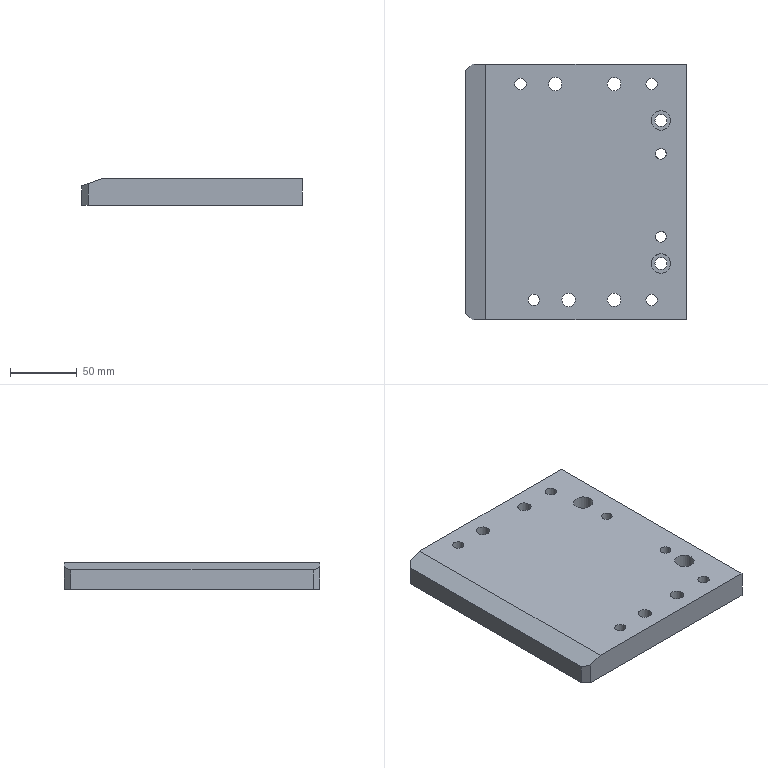Part | NX | features DIE-1 2 | 1 solid | 25 faces | box 165 x 191 x 20 mm | volume 604511 mm3 | cylinder 14 | plane 11 | commonest cylinder face diameters 8.506 x4 10 x4 8 x2 9.007 x2 14.5 x2
STEP:
#1=CARTESIAN_POINT('',(2183.347,-939.822,858.716));
#2=VERTEX_POINT('',#1);
#3=CARTESIAN_POINT('',(2179.094,-939.822,858.716));
#4=DIRECTION('',(0.,0.,-1.));
#5=DIRECTION('',(1.,0.,0.));
#6=AXIS2_PLACEMENT_3D('',#3,#4,#5);
#7=CIRCLE('',#6,4.253);
#8=EDGE_CURVE('',#2,#2,#7,.T.);
#9=ORIENTED_EDGE('',*,*,#8,.T.);
#10=EDGE_LOOP('',(#9));
#11=FACE_BOUND('',#10,.T.);
#12=CARTESIAN_POINT('',(2210.094,-939.822,858.716));
#13=VERTEX_POINT('',#12);
#14=CARTESIAN_POINT('',(2205.094,-939.822,858.716));
#15=DIRECTION('',(0.,0.,-1.));
#16=DIRECTION('',(1.,0.,0.));
#17=AXIS2_PLACEMENT_3D('',#14,#15,#16);
#18=CIRCLE('',#17,5.);
#19=EDGE_CURVE('',#13,#13,#18,.T.);
#20=ORIENTED_EDGE('',*,*,#19,.T.);
#21=EDGE_LOOP('',(#20));
#22=FACE_BOUND('',#21,.T.);
#23=CARTESIAN_POINT('',(2271.347,-939.822,858.716));
#24=VERTEX_POINT('',#23);
#25=CARTESIAN_POINT('',(2267.094,-939.822,858.716));
#26=DIRECTION('',(0.,0.,-1.));
#27=DIRECTION('',(1.,0.,0.));
#28=AXIS2_PLACEMENT_3D('',#25,#26,#27);
#29=CIRCLE('',#28,4.253);
#30=EDGE_CURVE('',#24,#24,#29,.T.);
#31=ORIENTED_EDGE('',*,*,#30,.T.);
#32=EDGE_LOOP('',(#31));
#33=FACE_BOUND('',#32,.T.);
#34=CARTESIAN_POINT('',(2244.094,-939.822,858.716));
#35=VERTEX_POINT('',#34);
#36=CARTESIAN_POINT('',(2239.094,-939.822,858.716));
#37=DIRECTION('',(0.,0.,-1.));
#38=DIRECTION('',(1.,0.,0.));
#39=AXIS2_PLACEMENT_3D('',#36,#37,#38);
#40=CIRCLE('',#39,5.);
#41=EDGE_CURVE('',#35,#35,#40,.T.);
#42=ORIENTED_EDGE('',*,*,#41,.T.);
#43=EDGE_LOOP('',(#42));
#44=FACE_BOUND('',#43,.T.);
#45=CARTESIAN_POINT('',(2173.347,-778.422,858.716));
#46=VERTEX_POINT('',#45);
#47=CARTESIAN_POINT('',(2169.094,-778.422,858.716));
#48=DIRECTION('',(0.,0.,-1.));
#49=DIRECTION('',(1.,0.,0.));
#50=AXIS2_PLACEMENT_3D('',#47,#48,#49);
#51=CIRCLE('',#50,4.253);
#52=EDGE_CURVE('',#46,#46,#51,.T.);
#53=ORIENTED_EDGE('',*,*,#52,.T.);
#54=EDGE_LOOP('',(#53));
#55=FACE_BOUND('',#54,.T.);
#56=CARTESIAN_POINT('',(2271.347,-778.422,858.716));
#57=VERTEX_POINT('',#56);
#58=CARTESIAN_POINT('',(2267.094,-778.422,858.716));
#59=DIRECTION('',(0.,0.,-1.));
#60=DIRECTION('',(1.,0.,0.));
#61=AXIS2_PLACEMENT_3D('',#58,#59,#60);
#62=CIRCLE('',#61,4.253);
#63=EDGE_CURVE('',#57,#57,#62,.T.);
#64=ORIENTED_EDGE('',*,*,#63,.T.);
#65=EDGE_LOOP('',(#64));
#66=FACE_BOUND('',#65,.T.);
#67=CARTESIAN_POINT('',(2200.094,-778.422,858.716));
#68=VERTEX_POINT('',#67);
#69=CARTESIAN_POINT('',(2195.094,-778.422,858.716));
#70=DIRECTION('',(0.,0.,-1.));
#71=DIRECTION('',(1.,0.,0.));
#72=AXIS2_PLACEMENT_3D('',#69,#70,#71);
#73=CIRCLE('',#72,5.);
#74=EDGE_CURVE('',#68,#68,#73,.T.);
#75=ORIENTED_EDGE('',*,*,#74,.T.);
#76=EDGE_LOOP('',(#75));
#77=FACE_BOUND('',#76,.T.);
#78=CARTESIAN_POINT('',(2244.094,-778.422,858.716));
#79=VERTEX_POINT('',#78);
#80=CARTESIAN_POINT('',(2239.094,-778.422,858.716));
#81=DIRECTION('',(0.,0.,-1.));
#82=DIRECTION('',(1.,0.,0.));
#83=AXIS2_PLACEMENT_3D('',#80,#81,#82);
#84=CIRCLE('',#83,5.);
#85=EDGE_CURVE('',#79,#79,#84,.T.);
#86=ORIENTED_EDGE('',*,*,#85,.T.);
#87=EDGE_LOOP('',(#86));
#88=FACE_BOUND('',#87,.T.);
#89=CARTESIAN_POINT('',(2281.344,-912.622,858.716));
#90=VERTEX_POINT('',#89);
#91=CARTESIAN_POINT('',(2274.094,-912.622,858.716));
#92=DIRECTION('',(0.,0.,1.));
#93=DIRECTION('',(1.,0.,0.));
#94=AXIS2_PLACEMENT_3D('',#91,#92,#93);
#95=CIRCLE('',#94,7.25);
#96=EDGE_CURVE('',#90,#90,#95,.F.);
#97=ORIENTED_EDGE('',*,*,#96,.T.);
#98=EDGE_LOOP('',(#97));
#99=FACE_BOUND('',#98,.T.);
#100=CARTESIAN_POINT('',(2278.094,-892.622,858.716));
#101=VERTEX_POINT('',#100);
#102=CARTESIAN_POINT('',(2274.094,-892.622,858.716));
#103=DIRECTION('',(0.,0.,-1.));
#104=DIRECTION('',(1.,0.,0.));
#105=AXIS2_PLACEMENT_3D('',#102,#103,#104);
#106=CIRCLE('',#105,4.);
#107=EDGE_CURVE('',#101,#101,#106,.T.);
#108=ORIENTED_EDGE('',*,*,#107,.T.);
#109=EDGE_LOOP('',(#108));
#110=FACE_BOUND('',#109,.T.);
#111=CARTESIAN_POINT('',(2278.094,-830.622,858.716));
#112=VERTEX_POINT('',#111);
#113=CARTESIAN_POINT('',(2274.094,-830.622,858.716));
#114=DIRECTION('',(0.,0.,-1.));
#115=DIRECTION('',(1.,0.,0.));
#116=AXIS2_PLACEMENT_3D('',#113,#114,#115);
#117=CIRCLE('',#116,4.);
#118=EDGE_CURVE('',#112,#112,#117,.T.);
#119=ORIENTED_EDGE('',*,*,#118,.T.);
#120=EDGE_LOOP('',(#119));
#121=FACE_BOUND('',#120,.T.);
#122=CARTESIAN_POINT('',(2281.344,-805.622,858.716));
#123=VERTEX_POINT('',#122);
#124=CARTESIAN_POINT('',(2274.094,-805.622,858.716));
#125=DIRECTION('',(0.,0.,1.));
#126=DIRECTION('',(1.,0.,0.));
#127=AXIS2_PLACEMENT_3D('',#124,#125,#126);
#128=CIRCLE('',#127,7.25);
#129=EDGE_CURVE('',#123,#123,#128,.F.);
#130=ORIENTED_EDGE('',*,*,#129,.T.);
#131=EDGE_LOOP('',(#130));
#132=FACE_BOUND('',#131,.T.);
#133=CARTESIAN_POINT('',(2293.094,-954.622,858.716));
#134=VERTEX_POINT('',#133);
#135=CARTESIAN_POINT('',(2143.094,-954.622,858.716));
#136=VERTEX_POINT('',#135);
#137=CARTESIAN_POINT('',(2118.094,-954.622,858.716));
#138=DIRECTION('',(-1.,0.,0.));
#139=VECTOR('',#138,1000.);
#140=LINE('',#137,#139);
#141=EDGE_CURVE('',#134,#136,#140,.T.);
#142=ORIENTED_EDGE('',*,*,#141,.F.);
#143=CARTESIAN_POINT('',(2293.094,-763.622,858.716));
#144=VERTEX_POINT('',#143);
#145=CARTESIAN_POINT('',(2293.094,-744.322,858.716));
#146=DIRECTION('',(0.,-1.,0.));
#147=VECTOR('',#146,1000.);
#148=LINE('',#145,#147);
#149=EDGE_CURVE('',#144,#134,#148,.T.);
#150=ORIENTED_EDGE('',*,*,#149,.F.);
#151=CARTESIAN_POINT('',(2143.094,-763.622,858.716));
#152=VERTEX_POINT('',#151);
#153=CARTESIAN_POINT('',(2293.094,-763.622,858.716));
#154=DIRECTION('',(1.,0.,0.));
#155=VECTOR('',#154,1000.);
#156=LINE('',#153,#155);
#157=EDGE_CURVE('',#152,#144,#156,.T.);
#158=ORIENTED_EDGE('',*,*,#157,.F.);
#159=CARTESIAN_POINT('',(2143.094,-830.822,858.716));
#160=DIRECTION('',(0.,-1.,0.));
#161=VECTOR('',#160,1000.);
#162=LINE('',#159,#161);
#163=EDGE_CURVE('',#152,#136,#162,.T.);
#164=ORIENTED_EDGE('',*,*,#163,.T.);
#165=EDGE_LOOP('',(#142,#150,#158,#164));
#166=FACE_BOUND('',#165,.T.);
#167=CARTESIAN_POINT('',(2203.862,-830.822,858.716));
#168=DIRECTION('',(0.,0.,1.));
#169=DIRECTION('',(-1.,0.,0.));
#170=AXIS2_PLACEMENT_3D('',#167,#168,#169);
#171=PLANE('',#170);
#172=ADVANCED_FACE('',(#11,#22,#33,#44,#55,#66,#77,#88,#99,#110,#121,#132,#166),#171,.T.);
#173=CARTESIAN_POINT('',(2183.347,-939.822,838.716));
#174=VERTEX_POINT('',#173);
#175=CARTESIAN_POINT('',(2179.094,-939.822,838.716));
#176=DIRECTION('',(0.,0.,1.));
#177=DIRECTION('',(1.,0.,0.));
#178=AXIS2_PLACEMENT_3D('',#175,#176,#177);
#179=CIRCLE('',#178,4.253);
#180=EDGE_CURVE('',#174,#174,#179,.T.);
#181=ORIENTED_EDGE('',*,*,#180,.T.);
#182=EDGE_LOOP('',(#181));
#183=FACE_BOUND('',#182,.T.);
#184=CARTESIAN_POINT('',(2210.094,-939.822,838.716));
#185=VERTEX_POINT('',#184);
#186=CARTESIAN_POINT('',(2205.094,-939.822,838.716));
#187=DIRECTION('',(0.,0.,1.));
#188=DIRECTION('',(1.,0.,0.));
#189=AXIS2_PLACEMENT_3D('',#186,#187,#188);
#190=CIRCLE('',#189,5.);
#191=EDGE_CURVE('',#185,#185,#190,.T.);
#192=ORIENTED_EDGE('',*,*,#191,.T.);
#193=EDGE_LOOP('',(#192));
#194=FACE_BOUND('',#193,.T.);
#195=CARTESIAN_POINT('',(2271.347,-939.822,838.716));
#196=VERTEX_POINT('',#195);
#197=CARTESIAN_POINT('',(2267.094,-939.822,838.716));
#198=DIRECTION('',(0.,0.,1.));
#199=DIRECTION('',(1.,0.,0.));
#200=AXIS2_PLACEMENT_3D('',#197,#198,#199);
#201=CIRCLE('',#200,4.253);
#202=EDGE_CURVE('',#196,#196,#201,.T.);
#203=ORIENTED_EDGE('',*,*,#202,.T.);
#204=EDGE_LOOP('',(#203));
#205=FACE_BOUND('',#204,.T.);
#206=CARTESIAN_POINT('',(2244.094,-939.822,838.716));
#207=VERTEX_POINT('',#206);
#208=CARTESIAN_POINT('',(2239.094,-939.822,838.716));
#209=DIRECTION('',(0.,0.,1.));
#210=DIRECTION('',(1.,0.,0.));
#211=AXIS2_PLACEMENT_3D('',#208,#209,#210);
#212=CIRCLE('',#211,5.);
#213=EDGE_CURVE('',#207,#207,#212,.T.);
#214=ORIENTED_EDGE('',*,*,#213,.T.);
#215=EDGE_LOOP('',(#214));
#216=FACE_BOUND('',#215,.T.);
#217=CARTESIAN_POINT('',(2173.347,-778.422,838.716));
#218=VERTEX_POINT('',#217);
#219=CARTESIAN_POINT('',(2169.094,-778.422,838.716));
#220=DIRECTION('',(0.,0.,1.));
#221=DIRECTION('',(1.,0.,0.));
#222=AXIS2_PLACEMENT_3D('',#219,#220,#221);
#223=CIRCLE('',#222,4.253);
#224=EDGE_CURVE('',#218,#218,#223,.T.);
#225=ORIENTED_EDGE('',*,*,#224,.T.);
#226=EDGE_LOOP('',(#225));
#227=FACE_BOUND('',#226,.T.);
#228=CARTESIAN_POINT('',(2271.347,-778.422,838.716));
#229=VERTEX_POINT('',#228);
#230=CARTESIAN_POINT('',(2267.094,-778.422,838.716));
#231=DIRECTION('',(0.,0.,1.));
#232=DIRECTION('',(1.,0.,0.));
#233=AXIS2_PLACEMENT_3D('',#230,#231,#232);
#234=CIRCLE('',#233,4.253);
#235=EDGE_CURVE('',#229,#229,#234,.T.);
#236=ORIENTED_EDGE('',*,*,#235,.T.);
#237=EDGE_LOOP('',(#236));
#238=FACE_BOUND('',#237,.T.);
#239=CARTESIAN_POINT('',(2200.094,-778.422,838.716));
#240=VERTEX_POINT('',#239);
#241=CARTESIAN_POINT('',(2195.094,-778.422,838.716));
#242=DIRECTION('',(0.,0.,1.));
#243=DIRECTION('',(1.,0.,0.));
#244=AXIS2_PLACEMENT_3D('',#241,#242,#243);
#245=CIRCLE('',#244,5.);
#246=EDGE_CURVE('',#240,#240,#245,.T.);
#247=ORIENTED_EDGE('',*,*,#246,.T.);
#248=EDGE_LOOP('',(#247));
#249=FACE_BOUND('',#248,.T.);
#250=CARTESIAN_POINT('',(2244.094,-778.422,838.716));
#251=VERTEX_POINT('',#250);
#252=CARTESIAN_POINT('',(2239.094,-778.422,838.716));
#253=DIRECTION('',(0.,0.,1.));
#254=DIRECTION('',(1.,0.,0.));
#255=AXIS2_PLACEMENT_3D('',#252,#253,#254);
#256=CIRCLE('',#255,5.);
#257=EDGE_CURVE('',#251,#251,#256,.T.);
#258=ORIENTED_EDGE('',*,*,#257,.T.);
#259=EDGE_LOOP('',(#258));
#260=FACE_BOUND('',#259,.T.);
#261=CARTESIAN_POINT('',(2278.597,-912.622,838.716));
#262=VERTEX_POINT('',#261);
#263=CARTESIAN_POINT('',(2274.094,-912.622,838.716));
#264=DIRECTION('',(0.,0.,1.));
#265=DIRECTION('',(1.,0.,0.));
#266=AXIS2_PLACEMENT_3D('',#263,#264,#265);
#267=CIRCLE('',#266,4.503);
#268=EDGE_CURVE('',#262,#262,#267,.F.);
#269=ORIENTED_EDGE('',*,*,#268,.F.);
#270=EDGE_LOOP('',(#269));
#271=FACE_BOUND('',#270,.T.);
#272=CARTESIAN_POINT('',(2274.094,-888.622,838.716));
#273=VERTEX_POINT('',#272);
#274=CARTESIAN_POINT('',(2274.094,-892.622,838.716));
#275=DIRECTION('',(0.,0.,-1.));
#276=DIRECTION('',(0.,1.,0.));
#277=AXIS2_PLACEMENT_3D('',#274,#275,#276);
#278=CIRCLE('',#277,4.);
#279=EDGE_CURVE('',#273,#273,#278,.T.);
#280=ORIENTED_EDGE('',*,*,#279,.F.);
#281=EDGE_LOOP('',(#280));
#282=FACE_BOUND('',#281,.T.);
#283=CARTESIAN_POINT('',(2274.094,-826.622,838.716));
#284=VERTEX_POINT('',#283);
#285=CARTESIAN_POINT('',(2274.094,-830.622,838.716));
#286=DIRECTION('',(0.,0.,-1.));
#287=DIRECTION('',(0.,1.,0.));
#288=AXIS2_PLACEMENT_3D('',#285,#286,#287);
#289=CIRCLE('',#288,4.);
#290=EDGE_CURVE('',#284,#284,#289,.T.);
#291=ORIENTED_EDGE('',*,*,#290,.F.);
#292=EDGE_LOOP('',(#291));
#293=FACE_BOUND('',#292,.T.);
#294=CARTESIAN_POINT('',(2278.597,-805.622,838.716));
#295=VERTEX_POINT('',#294);
#296=CARTESIAN_POINT('',(2274.094,-805.622,838.716));
#297=DIRECTION('',(0.,0.,1.));
#298=DIRECTION('',(1.,0.,0.));
#299=AXIS2_PLACEMENT_3D('',#296,#297,#298);
#300=CIRCLE('',#299,4.503);
#301=EDGE_CURVE('',#295,#295,#300,.F.);
#302=ORIENTED_EDGE('',*,*,#301,.F.);
#303=EDGE_LOOP('',(#302));
#304=FACE_BOUND('',#303,.T.);
#305=CARTESIAN_POINT('',(2293.094,-763.622,838.716));
#306=VERTEX_POINT('',#305);
#307=CARTESIAN_POINT('',(2132.894,-763.622,838.716));
#308=VERTEX_POINT('',#307);
#309=CARTESIAN_POINT('',(2203.862,-763.622,838.716));
#310=DIRECTION('',(-1.,0.,0.));
#311=VECTOR('',#310,1000.);
#312=LINE('',#309,#311);
#313=EDGE_CURVE('',#306,#308,#312,.T.);
#314=ORIENTED_EDGE('',*,*,#313,.F.);
#315=CARTESIAN_POINT('',(2293.094,-954.622,838.716));
#316=VERTEX_POINT('',#315);
#317=CARTESIAN_POINT('',(2293.094,-744.322,838.716));
#318=DIRECTION('',(0.,1.,0.));
#319=VECTOR('',#318,1000.);
#320=LINE('',#317,#319);
#321=EDGE_CURVE('',#316,#306,#320,.T.);
#322=ORIENTED_EDGE('',*,*,#321,.F.);
#323=CARTESIAN_POINT('',(2132.894,-954.622,838.716));
#324=VERTEX_POINT('',#323);
#325=CARTESIAN_POINT('',(2203.862,-954.622,838.716));
#326=DIRECTION('',(1.,0.,0.));
#327=VECTOR('',#326,1000.);
#328=LINE('',#325,#327);
#329=EDGE_CURVE('',#324,#316,#328,.T.);
#330=ORIENTED_EDGE('',*,*,#329,.F.);
#331=CARTESIAN_POINT('',(2128.094,-949.822,838.716));
#332=VERTEX_POINT('',#331);
#333=CARTESIAN_POINT('',(2128.094,-949.822,838.716));
#334=DIRECTION('',(-0.7071,0.7071,0.));
#335=VECTOR('',#334,1000.);
#336=LINE('',#333,#335);
#337=EDGE_CURVE('',#324,#332,#336,.T.);
#338=ORIENTED_EDGE('',*,*,#337,.T.);
#339=CARTESIAN_POINT('',(2128.094,-768.422,838.716));
#340=VERTEX_POINT('',#339);
#341=CARTESIAN_POINT('',(2128.094,-912.322,838.716));
#342=DIRECTION('',(0.,-1.,0.));
#343=VECTOR('',#342,1000.);
#344=LINE('',#341,#343);
#345=EDGE_CURVE('',#340,#332,#344,.T.);
#346=ORIENTED_EDGE('',*,*,#345,.F.);
#347=CARTESIAN_POINT('',(2128.094,-768.422,838.716));
#348=DIRECTION('',(-0.7071,-0.7071,0.));
#349=VECTOR('',#348,1000.);
#350=LINE('',#347,#349);
#351=EDGE_CURVE('',#308,#340,#350,.T.);
#352=ORIENTED_EDGE('',*,*,#351,.F.);
#353=EDGE_LOOP('',(#314,#322,#330,#338,#346,#352));
#354=FACE_BOUND('',#353,.T.);
#355=CARTESIAN_POINT('',(2203.862,-830.822,838.716));
#356=DIRECTION('',(0.,0.,1.));
#357=DIRECTION('',(-1.,0.,0.));
#358=AXIS2_PLACEMENT_3D('',#355,#356,#357);
#359=PLANE('',#358);
#360=ADVANCED_FACE('',(#183,#194,#205,#216,#227,#238,#249,#260,#271,#282,#293,#304,#354),#359,.F.);
#361=ORIENTED_EDGE('',*,*,#321,.T.);
#362=CARTESIAN_POINT('',(2293.094,-763.622,858.716));
#363=DIRECTION('',(0.,0.,-1.));
#364=VECTOR('',#363,1000.);
#365=LINE('',#362,#364);
#366=EDGE_CURVE('',#144,#306,#365,.T.);
#367=ORIENTED_EDGE('',*,*,#366,.F.);
#368=ORIENTED_EDGE('',*,*,#149,.T.);
#369=CARTESIAN_POINT('',(2293.094,-954.622,858.716));
#370=DIRECTION('',(0.,0.,-1.));
#371=VECTOR('',#370,1000.);
#372=LINE('',#369,#371);
#373=EDGE_CURVE('',#134,#316,#372,.T.);
#374=ORIENTED_EDGE('',*,*,#373,.T.);
#375=EDGE_LOOP('',(#361,#367,#368,#374));
#376=FACE_BOUND('',#375,.T.);
#377=CARTESIAN_POINT('',(2293.094,-917.322,858.716));
#378=DIRECTION('',(1.,0.,0.));
#379=DIRECTION('',(0.,0.,1.));
#380=AXIS2_PLACEMENT_3D('',#377,#378,#379);
#381=PLANE('',#380);
#382=ADVANCED_FACE('',(#376),#381,.T.);
#383=CARTESIAN_POINT('',(2132.894,-763.622,855.004));
#384=VERTEX_POINT('',#383);
#385=CARTESIAN_POINT('',(2132.894,-763.622,858.716));
#386=DIRECTION('',(0.,0.,-1.));
#387=VECTOR('',#386,1000.);
#388=LINE('',#385,#387);
#389=EDGE_CURVE('',#384,#308,#388,.T.);
#390=ORIENTED_EDGE('',*,*,#389,.F.);
#391=CARTESIAN_POINT('',(2275.547,-763.622,906.925));
#392=DIRECTION('',(0.9397,0.,0.342));
#393=VECTOR('',#392,1000.);
#394=LINE('',#391,#393);
#395=EDGE_CURVE('',#384,#152,#394,.T.);
#396=ORIENTED_EDGE('',*,*,#395,.T.);
#397=ORIENTED_EDGE('',*,*,#157,.T.);
#398=ORIENTED_EDGE('',*,*,#366,.T.);
#399=ORIENTED_EDGE('',*,*,#313,.T.);
#400=EDGE_LOOP('',(#390,#396,#397,#398,#399));
#401=FACE_BOUND('',#400,.T.);
#402=CARTESIAN_POINT('',(2293.094,-763.622,858.716));
#403=DIRECTION('',(0.,1.,0.));
#404=DIRECTION('',(0.,0.,-1.));
#405=AXIS2_PLACEMENT_3D('',#402,#403,#404);
#406=PLANE('',#405);
#407=ADVANCED_FACE('',(#401),#406,.T.);
#408=CARTESIAN_POINT('',(2128.094,-768.422,853.257));
#409=VERTEX_POINT('',#408);
#410=CARTESIAN_POINT('',(2128.094,-768.422,858.716));
#411=DIRECTION('',(0.,0.,-1.));
#412=VECTOR('',#411,1000.);
#413=LINE('',#410,#412);
#414=EDGE_CURVE('',#409,#340,#413,.T.);
#415=ORIENTED_EDGE('',*,*,#414,.F.);
#416=CARTESIAN_POINT('',(2133.715,-762.801,855.303));
#417=DIRECTION('',(0.6848,0.6848,0.2492));
#418=VECTOR('',#417,1000.);
#419=LINE('',#416,#418);
#420=EDGE_CURVE('',#409,#384,#419,.T.);
#421=ORIENTED_EDGE('',*,*,#420,.T.);
#422=ORIENTED_EDGE('',*,*,#389,.T.);
#423=ORIENTED_EDGE('',*,*,#351,.T.);
#424=EDGE_LOOP('',(#415,#421,#422,#423));
#425=FACE_BOUND('',#424,.T.);
#426=CARTESIAN_POINT('',(2133.094,-763.422,858.716));
#427=DIRECTION('',(-0.7071,0.7071,0.));
#428=DIRECTION('',(0.,0.,-1.));
#429=AXIS2_PLACEMENT_3D('',#426,#427,#428);
#430=PLANE('',#429);
#431=ADVANCED_FACE('',(#425),#430,.T.);
#432=ORIENTED_EDGE('',*,*,#345,.T.);
#433=CARTESIAN_POINT('',(2128.094,-949.822,853.257));
#434=VERTEX_POINT('',#433);
#435=CARTESIAN_POINT('',(2128.094,-949.822,858.716));
#436=DIRECTION('',(0.,0.,1.));
#437=VECTOR('',#436,1000.);
#438=LINE('',#435,#437);
#439=EDGE_CURVE('',#332,#434,#438,.T.);
#440=ORIENTED_EDGE('',*,*,#439,.T.);
#441=CARTESIAN_POINT('',(2128.094,-749.322,853.257));
#442=DIRECTION('',(0.,1.,0.));
#443=VECTOR('',#442,1000.);
#444=LINE('',#441,#443);
#445=EDGE_CURVE('',#434,#409,#444,.T.);
#446=ORIENTED_EDGE('',*,*,#445,.T.);
#447=ORIENTED_EDGE('',*,*,#414,.T.);
#448=EDGE_LOOP('',(#432,#440,#446,#447));
#449=FACE_BOUND('',#448,.T.);
#450=CARTESIAN_POINT('',(2128.094,-749.322,858.716));
#451=DIRECTION('',(-1.,0.,0.));
#452=DIRECTION('',(0.,0.,-1.));
#453=AXIS2_PLACEMENT_3D('',#450,#451,#452);
#454=PLANE('',#453);
#455=ADVANCED_FACE('',(#449),#454,.T.);
#456=ORIENTED_EDGE('',*,*,#420,.F.);
#457=ORIENTED_EDGE('',*,*,#445,.F.);
#458=CARTESIAN_POINT('',(2132.894,-954.622,855.004));
#459=VERTEX_POINT('',#458);
#460=CARTESIAN_POINT('',(2043.685,-865.413,822.534));
#461=DIRECTION('',(0.6848,-0.6848,0.2492));
#462=VECTOR('',#461,1000.);
#463=LINE('',#460,#462);
#464=EDGE_CURVE('',#434,#459,#463,.T.);
#465=ORIENTED_EDGE('',*,*,#464,.T.);
#466=CARTESIAN_POINT('',(2121.018,-954.622,850.681));
#467=DIRECTION('',(-0.9397,0.,-0.342));
#468=VECTOR('',#467,1000.);
#469=LINE('',#466,#468);
#470=EDGE_CURVE('',#136,#459,#469,.T.);
#471=ORIENTED_EDGE('',*,*,#470,.F.);
#472=ORIENTED_EDGE('',*,*,#163,.F.);
#473=ORIENTED_EDGE('',*,*,#395,.F.);
#474=EDGE_LOOP('',(#456,#457,#465,#471,#472,#473));
#475=FACE_BOUND('',#474,.T.);
#476=CARTESIAN_POINT('',(2128.094,-749.322,853.257));
#477=DIRECTION('',(0.342,0.,-0.9397));
#478=DIRECTION('',(0.,-1.,0.));
#479=AXIS2_PLACEMENT_3D('',#476,#477,#478);
#480=PLANE('',#479);
#481=ADVANCED_FACE('',(#475),#480,.F.);
#482=ORIENTED_EDGE('',*,*,#470,.T.);
#483=CARTESIAN_POINT('',(2132.894,-954.622,858.716));
#484=DIRECTION('',(0.,0.,-1.));
#485=VECTOR('',#484,1000.);
#486=LINE('',#483,#485);
#487=EDGE_CURVE('',#459,#324,#486,.T.);
#488=ORIENTED_EDGE('',*,*,#487,.T.);
#489=ORIENTED_EDGE('',*,*,#329,.T.);
#490=ORIENTED_EDGE('',*,*,#373,.F.);
#491=ORIENTED_EDGE('',*,*,#141,.T.);
#492=EDGE_LOOP('',(#482,#488,#489,#490,#491));
#493=FACE_BOUND('',#492,.T.);
#494=CARTESIAN_POINT('',(2118.094,-954.622,858.716));
#495=DIRECTION('',(0.,-1.,0.));
#496=DIRECTION('',(0.,0.,1.));
#497=AXIS2_PLACEMENT_3D('',#494,#495,#496);
#498=PLANE('',#497);
#499=ADVANCED_FACE('',(#493),#498,.T.);
#500=ORIENTED_EDGE('',*,*,#337,.F.);
#501=ORIENTED_EDGE('',*,*,#487,.F.);
#502=ORIENTED_EDGE('',*,*,#464,.F.);
#503=ORIENTED_EDGE('',*,*,#439,.F.);
#504=EDGE_LOOP('',(#500,#501,#502,#503));
#505=FACE_BOUND('',#504,.T.);
#506=CARTESIAN_POINT('',(2128.094,-949.822,858.716));
#507=DIRECTION('',(0.7071,0.7071,0.));
#508=DIRECTION('',(0.,0.,-1.));
#509=AXIS2_PLACEMENT_3D('',#506,#507,#508);
#510=PLANE('',#509);
#511=ADVANCED_FACE('',(#505),#510,.F.);
#512=CARTESIAN_POINT('',(2269.59,-805.622,847.716));
#513=VERTEX_POINT('',#512);
#514=CARTESIAN_POINT('',(2274.094,-805.622,847.716));
#515=DIRECTION('',(0.,0.,-1.));
#516=DIRECTION('',(-1.,0.,0.));
#517=AXIS2_PLACEMENT_3D('',#514,#515,#516);
#518=CIRCLE('',#517,4.503);
#519=EDGE_CURVE('',#513,#513,#518,.F.);
#520=ORIENTED_EDGE('',*,*,#519,.T.);
#521=EDGE_LOOP('',(#520));
#522=FACE_BOUND('',#521,.T.);
#523=ORIENTED_EDGE('',*,*,#301,.T.);
#524=EDGE_LOOP('',(#523));
#525=FACE_BOUND('',#524,.T.);
#526=CARTESIAN_POINT('',(2274.094,-805.622,838.716));
#527=DIRECTION('',(0.,0.,1.));
#528=DIRECTION('',(-1.,0.,0.));
#529=AXIS2_PLACEMENT_3D('',#526,#527,#528);
#530=CYLINDRICAL_SURFACE('',#529,4.503);
#531=ADVANCED_FACE('',(#522,#525),#530,.F.);
#532=ORIENTED_EDGE('',*,*,#129,.F.);
#533=EDGE_LOOP('',(#532));
#534=FACE_BOUND('',#533,.T.);
#535=CARTESIAN_POINT('',(2266.844,-805.622,847.716));
#536=VERTEX_POINT('',#535);
#537=CARTESIAN_POINT('',(2274.094,-805.622,847.716));
#538=DIRECTION('',(0.,0.,-1.));
#539=DIRECTION('',(-1.,0.,0.));
#540=AXIS2_PLACEMENT_3D('',#537,#538,#539);
#541=CIRCLE('',#540,7.25);
#542=EDGE_CURVE('',#536,#536,#541,.F.);
#543=ORIENTED_EDGE('',*,*,#542,.F.);
#544=EDGE_LOOP('',(#543));
#545=FACE_BOUND('',#544,.T.);
#546=CARTESIAN_POINT('',(2274.094,-805.622,847.716));
#547=DIRECTION('',(0.,0.,1.));
#548=DIRECTION('',(-1.,0.,0.));
#549=AXIS2_PLACEMENT_3D('',#546,#547,#548);
#550=CYLINDRICAL_SURFACE('',#549,7.25);
#551=ADVANCED_FACE('',(#534,#545),#550,.F.);
#552=ORIENTED_EDGE('',*,*,#519,.F.);
#553=EDGE_LOOP('',(#552));
#554=FACE_BOUND('',#553,.T.);
#555=ORIENTED_EDGE('',*,*,#542,.T.);
#556=EDGE_LOOP('',(#555));
#557=FACE_BOUND('',#556,.T.);
#558=CARTESIAN_POINT('',(2274.094,-805.622,847.716));
#559=DIRECTION('',(0.,0.,-1.));
#560=DIRECTION('',(1.,0.,0.));
#561=AXIS2_PLACEMENT_3D('',#558,#559,#560);
#562=PLANE('',#561);
#563=ADVANCED_FACE('',(#554,#557),#562,.F.);
#564=ORIENTED_EDGE('',*,*,#118,.F.);
#565=EDGE_LOOP('',(#564));
#566=FACE_BOUND('',#565,.T.);
#567=ORIENTED_EDGE('',*,*,#290,.T.);
#568=EDGE_LOOP('',(#567));
#569=FACE_BOUND('',#568,.T.);
#570=CARTESIAN_POINT('',(2274.094,-830.622,838.716));
#571=DIRECTION('',(0.,0.,1.));
#572=DIRECTION('',(-1.,0.,0.));
#573=AXIS2_PLACEMENT_3D('',#570,#571,#572);
#574=CYLINDRICAL_SURFACE('',#573,4.);
#575=ADVANCED_FACE('',(#566,#569),#574,.F.);
#576=ORIENTED_EDGE('',*,*,#107,.F.);
#577=EDGE_LOOP('',(#576));
#578=FACE_BOUND('',#577,.T.);
#579=ORIENTED_EDGE('',*,*,#279,.T.);
#580=EDGE_LOOP('',(#579));
#581=FACE_BOUND('',#580,.T.);
#582=CARTESIAN_POINT('',(2274.094,-892.622,838.716));
#583=DIRECTION('',(0.,0.,1.));
#584=DIRECTION('',(-1.,0.,0.));
#585=AXIS2_PLACEMENT_3D('',#582,#583,#584);
#586=CYLINDRICAL_SURFACE('',#585,4.);
#587=ADVANCED_FACE('',(#578,#581),#586,.F.);
#588=CARTESIAN_POINT('',(2269.59,-912.622,847.716));
#589=VERTEX_POINT('',#588);
#590=CARTESIAN_POINT('',(2274.094,-912.622,847.716));
#591=DIRECTION('',(0.,0.,-1.));
#592=DIRECTION('',(-1.,0.,0.));
#593=AXIS2_PLACEMENT_3D('',#590,#591,#592);
#594=CIRCLE('',#593,4.503);
#595=EDGE_CURVE('',#589,#589,#594,.F.);
#596=ORIENTED_EDGE('',*,*,#595,.T.);
#597=EDGE_LOOP('',(#596));
#598=FACE_BOUND('',#597,.T.);
#599=ORIENTED_EDGE('',*,*,#268,.T.);
#600=EDGE_LOOP('',(#599));
#601=FACE_BOUND('',#600,.T.);
#602=CARTESIAN_POINT('',(2274.094,-912.622,838.716));
#603=DIRECTION('',(0.,0.,1.));
#604=DIRECTION('',(-1.,0.,0.));
#605=AXIS2_PLACEMENT_3D('',#602,#603,#604);
#606=CYLINDRICAL_SURFACE('',#605,4.503);
#607=ADVANCED_FACE('',(#598,#601),#606,.F.);
#608=ORIENTED_EDGE('',*,*,#96,.F.);
#609=EDGE_LOOP('',(#608));
#610=FACE_BOUND('',#609,.T.);
#611=CARTESIAN_POINT('',(2266.844,-912.622,847.716));
#612=VERTEX_POINT('',#611);
#613=CARTESIAN_POINT('',(2274.094,-912.622,847.716));
#614=DIRECTION('',(0.,0.,-1.));
#615=DIRECTION('',(-1.,0.,0.));
#616=AXIS2_PLACEMENT_3D('',#613,#614,#615);
#617=CIRCLE('',#616,7.25);
#618=EDGE_CURVE('',#612,#612,#617,.F.);
#619=ORIENTED_EDGE('',*,*,#618,.F.);
#620=EDGE_LOOP('',(#619));
#621=FACE_BOUND('',#620,.T.);
#622=CARTESIAN_POINT('',(2274.094,-912.622,847.716));
#623=DIRECTION('',(0.,0.,1.));
#624=DIRECTION('',(-1.,0.,0.));
#625=AXIS2_PLACEMENT_3D('',#622,#623,#624);
#626=CYLINDRICAL_SURFACE('',#625,7.25);
#627=ADVANCED_FACE('',(#610,#621),#626,.F.);
#628=ORIENTED_EDGE('',*,*,#595,.F.);
#629=EDGE_LOOP('',(#628));
#630=FACE_BOUND('',#629,.T.);
#631=ORIENTED_EDGE('',*,*,#618,.T.);
#632=EDGE_LOOP('',(#631));
#633=FACE_BOUND('',#632,.T.);
#634=CARTESIAN_POINT('',(2274.094,-912.622,847.716));
#635=DIRECTION('',(0.,0.,-1.));
#636=DIRECTION('',(1.,0.,0.));
#637=AXIS2_PLACEMENT_3D('',#634,#635,#636);
#638=PLANE('',#637);
#639=ADVANCED_FACE('',(#630,#633),#638,.F.);
#640=ORIENTED_EDGE('',*,*,#85,.F.);
#641=EDGE_LOOP('',(#640));
#642=FACE_BOUND('',#641,.T.);
#643=ORIENTED_EDGE('',*,*,#257,.F.);
#644=EDGE_LOOP('',(#643));
#645=FACE_BOUND('',#644,.T.);
#646=CARTESIAN_POINT('',(2239.094,-778.422,858.716));
#647=DIRECTION('',(0.,0.,-1.));
#648=DIRECTION('',(1.,0.,0.));
#649=AXIS2_PLACEMENT_3D('',#646,#647,#648);
#650=CYLINDRICAL_SURFACE('',#649,5.);
#651=ADVANCED_FACE('',(#642,#645),#650,.F.);
#652=ORIENTED_EDGE('',*,*,#74,.F.);
#653=EDGE_LOOP('',(#652));
#654=FACE_BOUND('',#653,.T.);
#655=ORIENTED_EDGE('',*,*,#246,.F.);
#656=EDGE_LOOP('',(#655));
#657=FACE_BOUND('',#656,.T.);
#658=CARTESIAN_POINT('',(2195.094,-778.422,858.716));
#659=DIRECTION('',(0.,0.,-1.));
#660=DIRECTION('',(1.,0.,0.));
#661=AXIS2_PLACEMENT_3D('',#658,#659,#660);
#662=CYLINDRICAL_SURFACE('',#661,5.);
#663=ADVANCED_FACE('',(#654,#657),#662,.F.);
#664=ORIENTED_EDGE('',*,*,#63,.F.);
#665=EDGE_LOOP('',(#664));
#666=FACE_BOUND('',#665,.T.);
#667=ORIENTED_EDGE('',*,*,#235,.F.);
#668=EDGE_LOOP('',(#667));
#669=FACE_BOUND('',#668,.T.);
#670=CARTESIAN_POINT('',(2267.094,-778.422,858.716));
#671=DIRECTION('',(0.,0.,-1.));
#672=DIRECTION('',(1.,0.,0.));
#673=AXIS2_PLACEMENT_3D('',#670,#671,#672);
#674=CYLINDRICAL_SURFACE('',#673,4.253);
#675=ADVANCED_FACE('',(#666,#669),#674,.F.);
#676=ORIENTED_EDGE('',*,*,#52,.F.);
#677=EDGE_LOOP('',(#676));
#678=FACE_BOUND('',#677,.T.);
#679=ORIENTED_EDGE('',*,*,#224,.F.);
#680=EDGE_LOOP('',(#679));
#681=FACE_BOUND('',#680,.T.);
#682=CARTESIAN_POINT('',(2169.094,-778.422,858.716));
#683=DIRECTION('',(0.,0.,-1.));
#684=DIRECTION('',(1.,0.,0.));
#685=AXIS2_PLACEMENT_3D('',#682,#683,#684);
#686=CYLINDRICAL_SURFACE('',#685,4.253);
#687=ADVANCED_FACE('',(#678,#681),#686,.F.);
#688=ORIENTED_EDGE('',*,*,#41,.F.);
#689=EDGE_LOOP('',(#688));
#690=FACE_BOUND('',#689,.T.);
#691=ORIENTED_EDGE('',*,*,#213,.F.);
#692=EDGE_LOOP('',(#691));
#693=FACE_BOUND('',#692,.T.);
#694=CARTESIAN_POINT('',(2239.094,-939.822,858.716));
#695=DIRECTION('',(0.,0.,-1.));
#696=DIRECTION('',(1.,0.,0.));
#697=AXIS2_PLACEMENT_3D('',#694,#695,#696);
#698=CYLINDRICAL_SURFACE('',#697,5.);
#699=ADVANCED_FACE('',(#690,#693),#698,.F.);
#700=ORIENTED_EDGE('',*,*,#30,.F.);
#701=EDGE_LOOP('',(#700));
#702=FACE_BOUND('',#701,.T.);
#703=ORIENTED_EDGE('',*,*,#202,.F.);
#704=EDGE_LOOP('',(#703));
#705=FACE_BOUND('',#704,.T.);
#706=CARTESIAN_POINT('',(2267.094,-939.822,858.716));
#707=DIRECTION('',(0.,0.,-1.));
#708=DIRECTION('',(1.,0.,0.));
#709=AXIS2_PLACEMENT_3D('',#706,#707,#708);
#710=CYLINDRICAL_SURFACE('',#709,4.253);
#711=ADVANCED_FACE('',(#702,#705),#710,.F.);
#712=ORIENTED_EDGE('',*,*,#19,.F.);
#713=EDGE_LOOP('',(#712));
#714=FACE_BOUND('',#713,.T.);
#715=ORIENTED_EDGE('',*,*,#191,.F.);
#716=EDGE_LOOP('',(#715));
#717=FACE_BOUND('',#716,.T.);
#718=CARTESIAN_POINT('',(2205.094,-939.822,858.716));
#719=DIRECTION('',(0.,0.,-1.));
#720=DIRECTION('',(1.,0.,0.));
#721=AXIS2_PLACEMENT_3D('',#718,#719,#720);
#722=CYLINDRICAL_SURFACE('',#721,5.);
#723=ADVANCED_FACE('',(#714,#717),#722,.F.);
#724=ORIENTED_EDGE('',*,*,#8,.F.);
#725=EDGE_LOOP('',(#724));
#726=FACE_BOUND('',#725,.T.);
#727=ORIENTED_EDGE('',*,*,#180,.F.);
#728=EDGE_LOOP('',(#727));
#729=FACE_BOUND('',#728,.T.);
#730=CARTESIAN_POINT('',(2179.094,-939.822,858.716));
#731=DIRECTION('',(0.,0.,-1.));
#732=DIRECTION('',(1.,0.,0.));
#733=AXIS2_PLACEMENT_3D('',#730,#731,#732);
#734=CYLINDRICAL_SURFACE('',#733,4.253);
#735=ADVANCED_FACE('',(#726,#729),#734,.F.);
#736=CLOSED_SHELL('',(#172,#360,#382,#407,#431,#455,#481,#499,#511,#531,#551,#563,#575,#587,#607,#627,#639,#651,#663,#675,#687,#699,#711,#723,#735));
#737=MANIFOLD_SOLID_BREP('',#736);
#738=(LENGTH_UNIT()NAMED_UNIT(*)SI_UNIT(.MILLI.,.METRE.));
#739=UNCERTAINTY_MEASURE_WITH_UNIT(LENGTH_MEASURE(0.00001),#738,'','');
#740=(NAMED_UNIT(*)PLANE_ANGLE_UNIT()SI_UNIT($,.RADIAN.));
#741=(NAMED_UNIT(*)SI_UNIT($,.STERADIAN.)SOLID_ANGLE_UNIT());
#742=(GEOMETRIC_REPRESENTATION_CONTEXT(3)GLOBAL_UNCERTAINTY_ASSIGNED_CONTEXT((#739))GLOBAL_UNIT_ASSIGNED_CONTEXT((#738,#740,#741))REPRESENTATION_CONTEXT('',''));
#743=ADVANCED_BREP_SHAPE_REPRESENTATION('',(#737),#742);